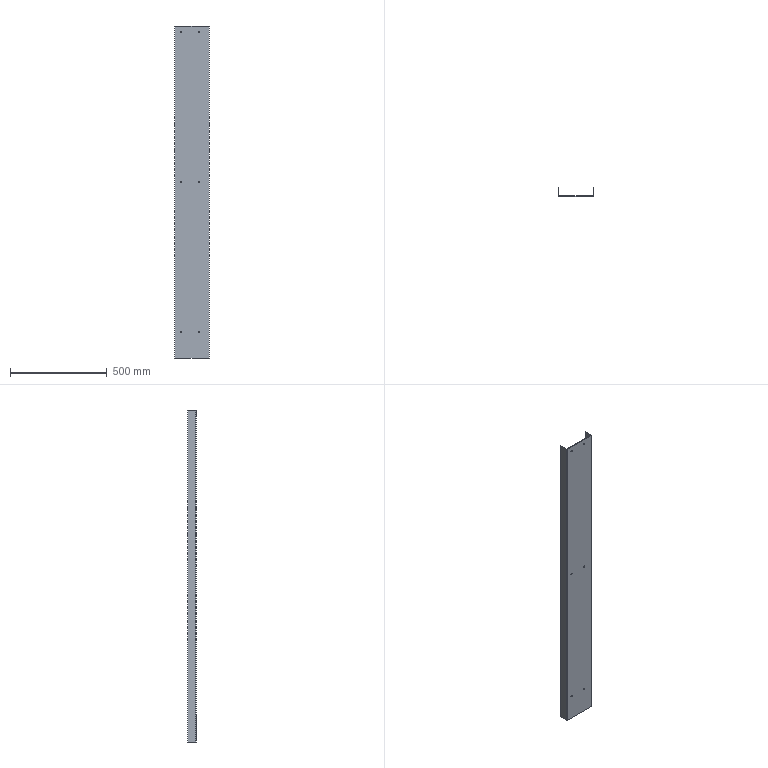Part | SolidWorks | features LPattern 2, Chamfer 1, FlatPattern 1, ICE 1, SMBaseFlange 1, SheetMetal 1 | 1 solid | 46 faces | box 180 x 45 x 1715 mm | volume 683780 mm3 | plane 18 | cylinder 16 | cone 12 | commonest cylinder face diameters 6 x12 1 x2 4 x2
STEP:
#1=CARTESIAN_POINT('',(85.039,61.658,-33.));
#2=VERTEX_POINT('',#1);
#3=CARTESIAN_POINT('',(85.039,61.658,-27.));
#4=VERTEX_POINT('',#3);
#5=CARTESIAN_POINT('',(85.039,61.658,-30.));
#6=DIRECTION('',(0.,1.,0.));
#7=DIRECTION('',(0.,0.,-1.));
#8=AXIS2_PLACEMENT_3D('',#5,#6,#7);
#9=CIRCLE('',#8,3.);
#10=EDGE_CURVE('',#2,#4,#9,.T.);
#11=ORIENTED_EDGE('',*,*,#10,.F.);
#12=CARTESIAN_POINT('',(85.039,62.658,-34.));
#13=VERTEX_POINT('',#12);
#14=CARTESIAN_POINT('',(85.039,61.658,-33.));
#15=DIRECTION('',(0.,0.7071,-0.7071));
#16=VECTOR('',#15,1000.);
#17=LINE('',#14,#16);
#18=EDGE_CURVE('',#2,#13,#17,.T.);
#19=ORIENTED_EDGE('',*,*,#18,.T.);
#20=CARTESIAN_POINT('',(85.039,62.658,-26.));
#21=VERTEX_POINT('',#20);
#22=CARTESIAN_POINT('',(85.039,62.658,-30.));
#23=DIRECTION('',(0.,-1.,0.));
#24=DIRECTION('',(0.,0.,-1.));
#25=AXIS2_PLACEMENT_3D('',#22,#23,#24);
#26=CIRCLE('',#25,4.);
#27=EDGE_CURVE('',#21,#13,#26,.T.);
#28=ORIENTED_EDGE('',*,*,#27,.F.);
#29=CARTESIAN_POINT('',(85.039,61.658,-27.));
#30=DIRECTION('',(0.,0.7071,0.7071));
#31=VECTOR('',#30,1000.);
#32=LINE('',#29,#31);
#33=EDGE_CURVE('',#4,#21,#32,.T.);
#34=ORIENTED_EDGE('',*,*,#33,.F.);
#35=EDGE_LOOP('',(#11,#19,#28,#34));
#36=FACE_OUTER_BOUND('',#35,.T.);
#37=CARTESIAN_POINT('',(85.039,61.658,-30.));
#38=DIRECTION('',(0.,1.,0.));
#39=DIRECTION('',(0.,0.,1.));
#40=AXIS2_PLACEMENT_3D('',#37,#38,#39);
#41=CONICAL_SURFACE('',#40,3.,0.7854);
#42=ADVANCED_FACE('',(#36),#41,.F.);
#43=CARTESIAN_POINT('',(-4.961,61.658,-33.));
#44=VERTEX_POINT('',#43);
#45=CARTESIAN_POINT('',(-4.961,61.658,-27.));
#46=VERTEX_POINT('',#45);
#47=CARTESIAN_POINT('',(-4.961,61.658,-30.));
#48=DIRECTION('',(0.,1.,0.));
#49=DIRECTION('',(0.,0.,-1.));
#50=AXIS2_PLACEMENT_3D('',#47,#48,#49);
#51=CIRCLE('',#50,3.);
#52=EDGE_CURVE('',#44,#46,#51,.T.);
#53=ORIENTED_EDGE('',*,*,#52,.F.);
#54=CARTESIAN_POINT('',(-4.961,62.658,-34.));
#55=VERTEX_POINT('',#54);
#56=CARTESIAN_POINT('',(-4.961,61.658,-33.));
#57=DIRECTION('',(0.,0.7071,-0.7071));
#58=VECTOR('',#57,1000.);
#59=LINE('',#56,#58);
#60=EDGE_CURVE('',#44,#55,#59,.T.);
#61=ORIENTED_EDGE('',*,*,#60,.T.);
#62=CARTESIAN_POINT('',(-4.961,62.658,-26.));
#63=VERTEX_POINT('',#62);
#64=CARTESIAN_POINT('',(-4.961,62.658,-30.));
#65=DIRECTION('',(0.,-1.,0.));
#66=DIRECTION('',(0.,0.,-1.));
#67=AXIS2_PLACEMENT_3D('',#64,#65,#66);
#68=CIRCLE('',#67,4.);
#69=EDGE_CURVE('',#63,#55,#68,.T.);
#70=ORIENTED_EDGE('',*,*,#69,.F.);
#71=CARTESIAN_POINT('',(-4.961,61.658,-27.));
#72=DIRECTION('',(0.,0.7071,0.7071));
#73=VECTOR('',#72,1000.);
#74=LINE('',#71,#73);
#75=EDGE_CURVE('',#46,#63,#74,.T.);
#76=ORIENTED_EDGE('',*,*,#75,.F.);
#77=EDGE_LOOP('',(#53,#61,#70,#76));
#78=FACE_OUTER_BOUND('',#77,.T.);
#79=CARTESIAN_POINT('',(-4.961,61.658,-30.));
#80=DIRECTION('',(0.,1.,0.));
#81=DIRECTION('',(0.,0.,1.));
#82=AXIS2_PLACEMENT_3D('',#79,#80,#81);
#83=CONICAL_SURFACE('',#82,3.,0.7854);
#84=ADVANCED_FACE('',(#78),#83,.F.);
#85=CARTESIAN_POINT('',(85.039,61.158,-27.));
#86=VERTEX_POINT('',#85);
#87=CARTESIAN_POINT('',(85.039,61.158,-33.));
#88=VERTEX_POINT('',#87);
#89=CARTESIAN_POINT('',(85.039,61.158,-30.));
#90=DIRECTION('',(0.,-1.,0.));
#91=DIRECTION('',(0.,0.,-1.));
#92=AXIS2_PLACEMENT_3D('',#89,#90,#91);
#93=CIRCLE('',#92,3.);
#94=EDGE_CURVE('',#86,#88,#93,.T.);
#95=ORIENTED_EDGE('',*,*,#94,.T.);
#96=CARTESIAN_POINT('',(85.039,52.658,-33.));
#97=DIRECTION('',(0.,1.,0.));
#98=VECTOR('',#97,1000.);
#99=LINE('',#96,#98);
#100=EDGE_CURVE('',#88,#2,#99,.T.);
#101=ORIENTED_EDGE('',*,*,#100,.T.);
#102=ORIENTED_EDGE('',*,*,#10,.T.);
#103=CARTESIAN_POINT('',(85.039,52.658,-27.));
#104=DIRECTION('',(0.,1.,0.));
#105=VECTOR('',#104,1000.);
#106=LINE('',#103,#105);
#107=EDGE_CURVE('',#86,#4,#106,.T.);
#108=ORIENTED_EDGE('',*,*,#107,.F.);
#109=EDGE_LOOP('',(#95,#101,#102,#108));
#110=FACE_OUTER_BOUND('',#109,.T.);
#111=CARTESIAN_POINT('',(85.039,52.658,-30.));
#112=DIRECTION('',(0.,1.,0.));
#113=DIRECTION('',(0.,0.,1.));
#114=AXIS2_PLACEMENT_3D('',#111,#112,#113);
#115=CYLINDRICAL_SURFACE('',#114,3.);
#116=ADVANCED_FACE('',(#110),#115,.F.);
#117=CARTESIAN_POINT('',(85.039,61.658,-808.));
#118=VERTEX_POINT('',#117);
#119=CARTESIAN_POINT('',(85.039,61.658,-802.));
#120=VERTEX_POINT('',#119);
#121=CARTESIAN_POINT('',(85.039,61.658,-805.));
#122=DIRECTION('',(0.,1.,0.));
#123=DIRECTION('',(0.,0.,-1.));
#124=AXIS2_PLACEMENT_3D('',#121,#122,#123);
#125=CIRCLE('',#124,3.);
#126=EDGE_CURVE('',#118,#120,#125,.T.);
#127=ORIENTED_EDGE('',*,*,#126,.F.);
#128=CARTESIAN_POINT('',(85.039,62.658,-809.));
#129=VERTEX_POINT('',#128);
#130=CARTESIAN_POINT('',(85.039,61.658,-808.));
#131=DIRECTION('',(0.,0.7071,-0.7071));
#132=VECTOR('',#131,1000.);
#133=LINE('',#130,#132);
#134=EDGE_CURVE('',#118,#129,#133,.T.);
#135=ORIENTED_EDGE('',*,*,#134,.T.);
#136=CARTESIAN_POINT('',(85.039,62.658,-801.));
#137=VERTEX_POINT('',#136);
#138=CARTESIAN_POINT('',(85.039,62.658,-805.));
#139=DIRECTION('',(0.,-1.,0.));
#140=DIRECTION('',(0.,0.,-1.));
#141=AXIS2_PLACEMENT_3D('',#138,#139,#140);
#142=CIRCLE('',#141,4.);
#143=EDGE_CURVE('',#137,#129,#142,.T.);
#144=ORIENTED_EDGE('',*,*,#143,.F.);
#145=CARTESIAN_POINT('',(85.039,61.658,-802.));
#146=DIRECTION('',(0.,0.7071,0.7071));
#147=VECTOR('',#146,1000.);
#148=LINE('',#145,#147);
#149=EDGE_CURVE('',#120,#137,#148,.T.);
#150=ORIENTED_EDGE('',*,*,#149,.F.);
#151=EDGE_LOOP('',(#127,#135,#144,#150));
#152=FACE_OUTER_BOUND('',#151,.T.);
#153=CARTESIAN_POINT('',(85.039,61.658,-805.));
#154=DIRECTION('',(0.,1.,0.));
#155=DIRECTION('',(0.,0.,1.));
#156=AXIS2_PLACEMENT_3D('',#153,#154,#155);
#157=CONICAL_SURFACE('',#156,3.,0.7854);
#158=ADVANCED_FACE('',(#152),#157,.F.);
#159=CARTESIAN_POINT('',(-4.961,61.658,-808.));
#160=VERTEX_POINT('',#159);
#161=CARTESIAN_POINT('',(-4.961,61.658,-802.));
#162=VERTEX_POINT('',#161);
#163=CARTESIAN_POINT('',(-4.961,61.658,-805.));
#164=DIRECTION('',(0.,1.,0.));
#165=DIRECTION('',(0.,0.,-1.));
#166=AXIS2_PLACEMENT_3D('',#163,#164,#165);
#167=CIRCLE('',#166,3.);
#168=EDGE_CURVE('',#160,#162,#167,.T.);
#169=ORIENTED_EDGE('',*,*,#168,.F.);
#170=CARTESIAN_POINT('',(-4.961,62.658,-809.));
#171=VERTEX_POINT('',#170);
#172=CARTESIAN_POINT('',(-4.961,61.658,-808.));
#173=DIRECTION('',(0.,0.7071,-0.7071));
#174=VECTOR('',#173,1000.);
#175=LINE('',#172,#174);
#176=EDGE_CURVE('',#160,#171,#175,.T.);
#177=ORIENTED_EDGE('',*,*,#176,.T.);
#178=CARTESIAN_POINT('',(-4.961,62.658,-801.));
#179=VERTEX_POINT('',#178);
#180=CARTESIAN_POINT('',(-4.961,62.658,-805.));
#181=DIRECTION('',(0.,-1.,0.));
#182=DIRECTION('',(0.,0.,-1.));
#183=AXIS2_PLACEMENT_3D('',#180,#181,#182);
#184=CIRCLE('',#183,4.);
#185=EDGE_CURVE('',#179,#171,#184,.T.);
#186=ORIENTED_EDGE('',*,*,#185,.F.);
#187=CARTESIAN_POINT('',(-4.961,61.658,-802.));
#188=DIRECTION('',(0.,0.7071,0.7071));
#189=VECTOR('',#188,1000.);
#190=LINE('',#187,#189);
#191=EDGE_CURVE('',#162,#179,#190,.T.);
#192=ORIENTED_EDGE('',*,*,#191,.F.);
#193=EDGE_LOOP('',(#169,#177,#186,#192));
#194=FACE_OUTER_BOUND('',#193,.T.);
#195=CARTESIAN_POINT('',(-4.961,61.658,-805.));
#196=DIRECTION('',(0.,1.,0.));
#197=DIRECTION('',(0.,0.,1.));
#198=AXIS2_PLACEMENT_3D('',#195,#196,#197);
#199=CONICAL_SURFACE('',#198,3.,0.7854);
#200=ADVANCED_FACE('',(#194),#199,.F.);
#201=CARTESIAN_POINT('',(85.039,61.158,-802.));
#202=VERTEX_POINT('',#201);
#203=CARTESIAN_POINT('',(85.039,61.158,-808.));
#204=VERTEX_POINT('',#203);
#205=CARTESIAN_POINT('',(85.039,61.158,-805.));
#206=DIRECTION('',(0.,-1.,0.));
#207=DIRECTION('',(0.,0.,-1.));
#208=AXIS2_PLACEMENT_3D('',#205,#206,#207);
#209=CIRCLE('',#208,3.);
#210=EDGE_CURVE('',#202,#204,#209,.T.);
#211=ORIENTED_EDGE('',*,*,#210,.T.);
#212=CARTESIAN_POINT('',(85.039,52.658,-808.));
#213=DIRECTION('',(0.,1.,0.));
#214=VECTOR('',#213,1000.);
#215=LINE('',#212,#214);
#216=EDGE_CURVE('',#204,#118,#215,.T.);
#217=ORIENTED_EDGE('',*,*,#216,.T.);
#218=ORIENTED_EDGE('',*,*,#126,.T.);
#219=CARTESIAN_POINT('',(85.039,52.658,-802.));
#220=DIRECTION('',(0.,1.,0.));
#221=VECTOR('',#220,1000.);
#222=LINE('',#219,#221);
#223=EDGE_CURVE('',#202,#120,#222,.T.);
#224=ORIENTED_EDGE('',*,*,#223,.F.);
#225=EDGE_LOOP('',(#211,#217,#218,#224));
#226=FACE_OUTER_BOUND('',#225,.T.);
#227=CARTESIAN_POINT('',(85.039,52.658,-805.));
#228=DIRECTION('',(0.,1.,0.));
#229=DIRECTION('',(0.,0.,1.));
#230=AXIS2_PLACEMENT_3D('',#227,#228,#229);
#231=CYLINDRICAL_SURFACE('',#230,3.);
#232=ADVANCED_FACE('',(#226),#231,.F.);
#233=CARTESIAN_POINT('',(-4.961,61.158,-27.));
#234=VERTEX_POINT('',#233);
#235=CARTESIAN_POINT('',(-4.961,61.158,-33.));
#236=VERTEX_POINT('',#235);
#237=CARTESIAN_POINT('',(-4.961,61.158,-30.));
#238=DIRECTION('',(0.,-1.,0.));
#239=DIRECTION('',(0.,0.,-1.));
#240=AXIS2_PLACEMENT_3D('',#237,#238,#239);
#241=CIRCLE('',#240,3.);
#242=EDGE_CURVE('',#234,#236,#241,.T.);
#243=ORIENTED_EDGE('',*,*,#242,.T.);
#244=CARTESIAN_POINT('',(-4.961,52.658,-33.));
#245=DIRECTION('',(0.,1.,0.));
#246=VECTOR('',#245,1000.);
#247=LINE('',#244,#246);
#248=EDGE_CURVE('',#236,#44,#247,.T.);
#249=ORIENTED_EDGE('',*,*,#248,.T.);
#250=ORIENTED_EDGE('',*,*,#52,.T.);
#251=CARTESIAN_POINT('',(-4.961,52.658,-27.));
#252=DIRECTION('',(0.,1.,0.));
#253=VECTOR('',#252,1000.);
#254=LINE('',#251,#253);
#255=EDGE_CURVE('',#234,#46,#254,.T.);
#256=ORIENTED_EDGE('',*,*,#255,.F.);
#257=EDGE_LOOP('',(#243,#249,#250,#256));
#258=FACE_OUTER_BOUND('',#257,.T.);
#259=CARTESIAN_POINT('',(-4.961,52.658,-30.));
#260=DIRECTION('',(0.,1.,0.));
#261=DIRECTION('',(0.,0.,1.));
#262=AXIS2_PLACEMENT_3D('',#259,#260,#261);
#263=CYLINDRICAL_SURFACE('',#262,3.);
#264=ADVANCED_FACE('',(#258),#263,.F.);
#265=CARTESIAN_POINT('',(-4.961,61.158,-802.));
#266=VERTEX_POINT('',#265);
#267=CARTESIAN_POINT('',(-4.961,61.158,-808.));
#268=VERTEX_POINT('',#267);
#269=CARTESIAN_POINT('',(-4.961,61.158,-805.));
#270=DIRECTION('',(0.,-1.,0.));
#271=DIRECTION('',(0.,0.,-1.));
#272=AXIS2_PLACEMENT_3D('',#269,#270,#271);
#273=CIRCLE('',#272,3.);
#274=EDGE_CURVE('',#266,#268,#273,.T.);
#275=ORIENTED_EDGE('',*,*,#274,.T.);
#276=CARTESIAN_POINT('',(-4.961,52.658,-808.));
#277=DIRECTION('',(0.,1.,0.));
#278=VECTOR('',#277,1000.);
#279=LINE('',#276,#278);
#280=EDGE_CURVE('',#268,#160,#279,.T.);
#281=ORIENTED_EDGE('',*,*,#280,.T.);
#282=ORIENTED_EDGE('',*,*,#168,.T.);
#283=CARTESIAN_POINT('',(-4.961,52.658,-802.));
#284=DIRECTION('',(0.,1.,0.));
#285=VECTOR('',#284,1000.);
#286=LINE('',#283,#285);
#287=EDGE_CURVE('',#266,#162,#286,.T.);
#288=ORIENTED_EDGE('',*,*,#287,.F.);
#289=EDGE_LOOP('',(#275,#281,#282,#288));
#290=FACE_OUTER_BOUND('',#289,.T.);
#291=CARTESIAN_POINT('',(-4.961,52.658,-805.));
#292=DIRECTION('',(0.,1.,0.));
#293=DIRECTION('',(0.,0.,1.));
#294=AXIS2_PLACEMENT_3D('',#291,#292,#293);
#295=CYLINDRICAL_SURFACE('',#294,3.);
#296=ADVANCED_FACE('',(#290),#295,.F.);
#297=CARTESIAN_POINT('',(85.039,61.658,-1583.));
#298=VERTEX_POINT('',#297);
#299=CARTESIAN_POINT('',(85.039,61.658,-1577.));
#300=VERTEX_POINT('',#299);
#301=CARTESIAN_POINT('',(85.039,61.658,-1580.));
#302=DIRECTION('',(0.,1.,0.));
#303=DIRECTION('',(0.,0.,-1.));
#304=AXIS2_PLACEMENT_3D('',#301,#302,#303);
#305=CIRCLE('',#304,3.);
#306=EDGE_CURVE('',#298,#300,#305,.T.);
#307=ORIENTED_EDGE('',*,*,#306,.F.);
#308=CARTESIAN_POINT('',(85.039,62.658,-1584.));
#309=VERTEX_POINT('',#308);
#310=CARTESIAN_POINT('',(85.039,61.658,-1583.));
#311=DIRECTION('',(0.,0.7071,-0.7071));
#312=VECTOR('',#311,1000.);
#313=LINE('',#310,#312);
#314=EDGE_CURVE('',#298,#309,#313,.T.);
#315=ORIENTED_EDGE('',*,*,#314,.T.);
#316=CARTESIAN_POINT('',(85.039,62.658,-1576.));
#317=VERTEX_POINT('',#316);
#318=CARTESIAN_POINT('',(85.039,62.658,-1580.));
#319=DIRECTION('',(0.,-1.,0.));
#320=DIRECTION('',(0.,0.,-1.));
#321=AXIS2_PLACEMENT_3D('',#318,#319,#320);
#322=CIRCLE('',#321,4.);
#323=EDGE_CURVE('',#317,#309,#322,.T.);
#324=ORIENTED_EDGE('',*,*,#323,.F.);
#325=CARTESIAN_POINT('',(85.039,61.658,-1577.));
#326=DIRECTION('',(0.,0.7071,0.7071));
#327=VECTOR('',#326,1000.);
#328=LINE('',#325,#327);
#329=EDGE_CURVE('',#300,#317,#328,.T.);
#330=ORIENTED_EDGE('',*,*,#329,.F.);
#331=EDGE_LOOP('',(#307,#315,#324,#330));
#332=FACE_OUTER_BOUND('',#331,.T.);
#333=CARTESIAN_POINT('',(85.039,61.658,-1580.));
#334=DIRECTION('',(0.,1.,0.));
#335=DIRECTION('',(0.,0.,1.));
#336=AXIS2_PLACEMENT_3D('',#333,#334,#335);
#337=CONICAL_SURFACE('',#336,3.,0.7854);
#338=ADVANCED_FACE('',(#332),#337,.F.);
#339=CARTESIAN_POINT('',(85.039,61.158,-1577.));
#340=VERTEX_POINT('',#339);
#341=CARTESIAN_POINT('',(85.039,61.158,-1583.));
#342=VERTEX_POINT('',#341);
#343=CARTESIAN_POINT('',(85.039,61.158,-1580.));
#344=DIRECTION('',(0.,-1.,0.));
#345=DIRECTION('',(0.,0.,-1.));
#346=AXIS2_PLACEMENT_3D('',#343,#344,#345);
#347=CIRCLE('',#346,3.);
#348=EDGE_CURVE('',#340,#342,#347,.T.);
#349=ORIENTED_EDGE('',*,*,#348,.T.);
#350=CARTESIAN_POINT('',(85.039,52.658,-1583.));
#351=DIRECTION('',(0.,1.,0.));
#352=VECTOR('',#351,1000.);
#353=LINE('',#350,#352);
#354=EDGE_CURVE('',#342,#298,#353,.T.);
#355=ORIENTED_EDGE('',*,*,#354,.T.);
#356=ORIENTED_EDGE('',*,*,#306,.T.);
#357=CARTESIAN_POINT('',(85.039,52.658,-1577.));
#358=DIRECTION('',(0.,1.,0.));
#359=VECTOR('',#358,1000.);
#360=LINE('',#357,#359);
#361=EDGE_CURVE('',#340,#300,#360,.T.);
#362=ORIENTED_EDGE('',*,*,#361,.F.);
#363=EDGE_LOOP('',(#349,#355,#356,#362));
#364=FACE_OUTER_BOUND('',#363,.T.);
#365=CARTESIAN_POINT('',(85.039,52.658,-1580.));
#366=DIRECTION('',(0.,1.,0.));
#367=DIRECTION('',(0.,0.,1.));
#368=AXIS2_PLACEMENT_3D('',#365,#366,#367);
#369=CYLINDRICAL_SURFACE('',#368,3.);
#370=ADVANCED_FACE('',(#364),#369,.F.);
#371=CARTESIAN_POINT('',(-4.961,61.658,-1583.));
#372=VERTEX_POINT('',#371);
#373=CARTESIAN_POINT('',(-4.961,61.658,-1577.));
#374=VERTEX_POINT('',#373);
#375=CARTESIAN_POINT('',(-4.961,61.658,-1580.));
#376=DIRECTION('',(0.,1.,0.));
#377=DIRECTION('',(0.,0.,-1.));
#378=AXIS2_PLACEMENT_3D('',#375,#376,#377);
#379=CIRCLE('',#378,3.);
#380=EDGE_CURVE('',#372,#374,#379,.T.);
#381=ORIENTED_EDGE('',*,*,#380,.F.);
#382=CARTESIAN_POINT('',(-4.961,62.658,-1584.));
#383=VERTEX_POINT('',#382);
#384=CARTESIAN_POINT('',(-4.961,61.658,-1583.));
#385=DIRECTION('',(0.,0.7071,-0.7071));
#386=VECTOR('',#385,1000.);
#387=LINE('',#384,#386);
#388=EDGE_CURVE('',#372,#383,#387,.T.);
#389=ORIENTED_EDGE('',*,*,#388,.T.);
#390=CARTESIAN_POINT('',(-4.961,62.658,-1576.));
#391=VERTEX_POINT('',#390);
#392=CARTESIAN_POINT('',(-4.961,62.658,-1580.));
#393=DIRECTION('',(0.,-1.,0.));
#394=DIRECTION('',(0.,0.,-1.));
#395=AXIS2_PLACEMENT_3D('',#392,#393,#394);
#396=CIRCLE('',#395,4.);
#397=EDGE_CURVE('',#391,#383,#396,.T.);
#398=ORIENTED_EDGE('',*,*,#397,.F.);
#399=CARTESIAN_POINT('',(-4.961,61.658,-1577.));
#400=DIRECTION('',(0.,0.7071,0.7071));
#401=VECTOR('',#400,1000.);
#402=LINE('',#399,#401);
#403=EDGE_CURVE('',#374,#391,#402,.T.);
#404=ORIENTED_EDGE('',*,*,#403,.F.);
#405=EDGE_LOOP('',(#381,#389,#398,#404));
#406=FACE_OUTER_BOUND('',#405,.T.);
#407=CARTESIAN_POINT('',(-4.961,61.658,-1580.));
#408=DIRECTION('',(0.,1.,0.));
#409=DIRECTION('',(0.,0.,1.));
#410=AXIS2_PLACEMENT_3D('',#407,#408,#409);
#411=CONICAL_SURFACE('',#410,3.,0.7854);
#412=ADVANCED_FACE('',(#406),#411,.F.);
#413=CARTESIAN_POINT('',(-4.961,61.158,-1577.));
#414=VERTEX_POINT('',#413);
#415=CARTESIAN_POINT('',(-4.961,61.158,-1583.));
#416=VERTEX_POINT('',#415);
#417=CARTESIAN_POINT('',(-4.961,61.158,-1580.));
#418=DIRECTION('',(0.,-1.,0.));
#419=DIRECTION('',(0.,0.,-1.));
#420=AXIS2_PLACEMENT_3D('',#417,#418,#419);
#421=CIRCLE('',#420,3.);
#422=EDGE_CURVE('',#414,#416,#421,.T.);
#423=ORIENTED_EDGE('',*,*,#422,.T.);
#424=CARTESIAN_POINT('',(-4.961,52.658,-1583.));
#425=DIRECTION('',(0.,1.,0.));
#426=VECTOR('',#425,1000.);
#427=LINE('',#424,#426);
#428=EDGE_CURVE('',#416,#372,#427,.T.);
#429=ORIENTED_EDGE('',*,*,#428,.T.);
#430=ORIENTED_EDGE('',*,*,#380,.T.);
#431=CARTESIAN_POINT('',(-4.961,52.658,-1577.));
#432=DIRECTION('',(0.,1.,0.));
#433=VECTOR('',#432,1000.);
#434=LINE('',#431,#433);
#435=EDGE_CURVE('',#414,#374,#434,.T.);
#436=ORIENTED_EDGE('',*,*,#435,.F.);
#437=EDGE_LOOP('',(#423,#429,#430,#436));
#438=FACE_OUTER_BOUND('',#437,.T.);
#439=CARTESIAN_POINT('',(-4.961,52.658,-1580.));
#440=DIRECTION('',(0.,1.,0.));
#441=DIRECTION('',(0.,0.,1.));
#442=AXIS2_PLACEMENT_3D('',#439,#440,#441);
#443=CYLINDRICAL_SURFACE('',#442,3.);
#444=ADVANCED_FACE('',(#438),#443,.F.);
#445=CARTESIAN_POINT('',(-37.961,61.158,-1715.));
#446=VERTEX_POINT('',#445);
#447=CARTESIAN_POINT('',(-37.961,62.658,-1715.));
#448=VERTEX_POINT('',#447);
#449=CARTESIAN_POINT('',(-37.961,61.158,-1715.));
#450=DIRECTION('',(0.,1.,0.));
#451=VECTOR('',#450,1000.);
#452=LINE('',#449,#451);
#453=EDGE_CURVE('',#446,#448,#452,.T.);
#454=ORIENTED_EDGE('',*,*,#453,.F.);
#455=CARTESIAN_POINT('',(-39.961,63.158,-1715.));
#456=VERTEX_POINT('',#455);
#457=CARTESIAN_POINT('',(-37.961,63.158,-1715.));
#458=DIRECTION('',(0.,0.,1.));
#459=DIRECTION('',(-1.,0.,0.));
#460=AXIS2_PLACEMENT_3D('',#457,#458,#459);
#461=CIRCLE('',#460,2.);
#462=EDGE_CURVE('',#456,#446,#461,.T.);
#463=ORIENTED_EDGE('',*,*,#462,.F.);
#464=CARTESIAN_POINT('',(-38.461,63.158,-1715.));
#465=VERTEX_POINT('',#464);
#466=CARTESIAN_POINT('',(-38.461,63.158,-1715.));
#467=DIRECTION('',(-1.,0.,0.));
#468=VECTOR('',#467,1000.);
#469=LINE('',#466,#468);
#470=EDGE_CURVE('',#465,#456,#469,.T.);
#471=ORIENTED_EDGE('',*,*,#470,.F.);
#472=CARTESIAN_POINT('',(-37.961,63.158,-1715.));
#473=DIRECTION('',(0.,0.,1.));
#474=DIRECTION('',(1.,0.,0.));
#475=AXIS2_PLACEMENT_3D('',#472,#473,#474);
#476=CIRCLE('',#475,0.5);
#477=EDGE_CURVE('',#465,#448,#476,.T.);
#478=ORIENTED_EDGE('',*,*,#477,.T.);
#479=EDGE_LOOP('',(#454,#463,#471,#478));
#480=FACE_OUTER_BOUND('',#479,.T.);
#481=CARTESIAN_POINT('',(-37.961,61.158,-1715.));
#482=DIRECTION('',(0.,0.,-1.));
#483=DIRECTION('',(-1.,0.,0.));
#484=AXIS2_PLACEMENT_3D('',#481,#482,#483);
#485=PLANE('',#484);
#486=ADVANCED_FACE('',(#480),#485,.T.);
#487=CARTESIAN_POINT('',(138.039,61.158,-1715.));
#488=VERTEX_POINT('',#487);
#489=CARTESIAN_POINT('',(-39.961,61.158,-1715.));
#490=DIRECTION('',(1.,0.,0.));
#491=VECTOR('',#490,1000.);
#492=LINE('',#489,#491);
#493=EDGE_CURVE('',#446,#488,#492,.T.);
#494=ORIENTED_EDGE('',*,*,#493,.F.);
#495=ORIENTED_EDGE('',*,*,#453,.T.);
#496=CARTESIAN_POINT('',(138.039,62.658,-1715.));
#497=VERTEX_POINT('',#496);
#498=CARTESIAN_POINT('',(-39.961,62.658,-1715.));
#499=DIRECTION('',(1.,0.,0.));
#500=VECTOR('',#499,1000.);
#501=LINE('',#498,#500);
#502=EDGE_CURVE('',#448,#497,#501,.T.);
#503=ORIENTED_EDGE('',*,*,#502,.T.);
#504=CARTESIAN_POINT('',(138.039,62.658,-1715.));
#505=DIRECTION('',(0.,-1.,0.));
#506=VECTOR('',#505,1000.);
#507=LINE('',#504,#506);
#508=EDGE_CURVE('',#497,#488,#507,.T.);
#509=ORIENTED_EDGE('',*,*,#508,.T.);
#510=EDGE_LOOP('',(#494,#495,#503,#509));
#511=FACE_OUTER_BOUND('',#510,.T.);
#512=CARTESIAN_POINT('',(-38.461,63.158,-1715.));
#513=DIRECTION('',(0.,0.,-1.));
#514=DIRECTION('',(-1.,0.,0.));
#515=AXIS2_PLACEMENT_3D('',#512,#513,#514);
#516=PLANE('',#515);
#517=ADVANCED_FACE('',(#511),#516,.T.);
#518=CARTESIAN_POINT('',(-39.961,63.158,0.));
#519=VERTEX_POINT('',#518);
#520=CARTESIAN_POINT('',(-38.461,63.158,0.));
#521=VERTEX_POINT('',#520);
#522=CARTESIAN_POINT('',(-39.961,63.158,0.));
#523=DIRECTION('',(1.,0.,0.));
#524=VECTOR('',#523,1000.);
#525=LINE('',#522,#524);
#526=EDGE_CURVE('',#519,#521,#525,.T.);
#527=ORIENTED_EDGE('',*,*,#526,.F.);
#528=CARTESIAN_POINT('',(-37.961,61.158,0.));
#529=VERTEX_POINT('',#528);
#530=CARTESIAN_POINT('',(-37.961,63.158,0.));
#531=DIRECTION('',(0.,0.,1.));
#532=DIRECTION('',(-1.,0.,0.));
#533=AXIS2_PLACEMENT_3D('',#530,#531,#532);
#534=CIRCLE('',#533,2.);
#535=EDGE_CURVE('',#519,#529,#534,.T.);
#536=ORIENTED_EDGE('',*,*,#535,.T.);
#537=CARTESIAN_POINT('',(-37.961,62.658,0.));
#538=VERTEX_POINT('',#537);
#539=CARTESIAN_POINT('',(-37.961,62.658,0.));
#540=DIRECTION('',(0.,-1.,0.));
#541=VECTOR('',#540,1000.);
#542=LINE('',#539,#541);
#543=EDGE_CURVE('',#538,#529,#542,.T.);
#544=ORIENTED_EDGE('',*,*,#543,.F.);
#545=CARTESIAN_POINT('',(-37.961,63.158,0.));
#546=DIRECTION('',(0.,0.,1.));
#547=DIRECTION('',(1.,0.,0.));
#548=AXIS2_PLACEMENT_3D('',#545,#546,#547);
#549=CIRCLE('',#548,0.5);
#550=EDGE_CURVE('',#521,#538,#549,.T.);
#551=ORIENTED_EDGE('',*,*,#550,.F.);
#552=EDGE_LOOP('',(#527,#536,#544,#551));
#553=FACE_OUTER_BOUND('',#552,.T.);
#554=CARTESIAN_POINT('',(-39.961,63.158,0.));
#555=DIRECTION('',(0.,0.,1.));
#556=DIRECTION('',(1.,0.,0.));
#557=AXIS2_PLACEMENT_3D('',#554,#555,#556);
#558=PLANE('',#557);
#559=ADVANCED_FACE('',(#553),#558,.T.);
#560=CARTESIAN_POINT('',(-39.961,106.158,0.));
#561=VERTEX_POINT('',#560);
#562=CARTESIAN_POINT('',(-39.961,106.158,0.));
#563=DIRECTION('',(0.,-1.,0.));
#564=VECTOR('',#563,1000.);
#565=LINE('',#562,#564);
#566=EDGE_CURVE('',#561,#519,#565,.T.);
#567=ORIENTED_EDGE('',*,*,#566,.T.);
#568=ORIENTED_EDGE('',*,*,#526,.T.);
#569=CARTESIAN_POINT('',(-38.461,106.158,0.));
#570=VERTEX_POINT('',#569);
#571=CARTESIAN_POINT('',(-38.461,106.158,0.));
#572=DIRECTION('',(0.,-1.,0.));
#573=VECTOR('',#572,1000.);
#574=LINE('',#571,#573);
#575=EDGE_CURVE('',#570,#521,#574,.T.);
#576=ORIENTED_EDGE('',*,*,#575,.F.);
#577=CARTESIAN_POINT('',(-39.961,106.158,0.));
#578=DIRECTION('',(1.,0.,0.));
#579=VECTOR('',#578,1000.);
#580=LINE('',#577,#579);
#581=EDGE_CURVE('',#561,#570,#580,.T.);
#582=ORIENTED_EDGE('',*,*,#581,.F.);
#583=EDGE_LOOP('',(#567,#568,#576,#582));
#584=FACE_OUTER_BOUND('',#583,.T.);
#585=CARTESIAN_POINT('',(-37.961,62.658,0.));
#586=DIRECTION('',(0.,0.,1.));
#587=DIRECTION('',(1.,0.,0.));
#588=AXIS2_PLACEMENT_3D('',#585,#586,#587);
#589=PLANE('',#588);
#590=ADVANCED_FACE('',(#584),#589,.T.);
#591=CARTESIAN_POINT('',(140.039,63.158,-1715.));
#592=VERTEX_POINT('',#591);
#593=CARTESIAN_POINT('',(138.539,63.158,-1715.));
#594=VERTEX_POINT('',#593);
#595=CARTESIAN_POINT('',(140.039,63.158,-1715.));
#596=DIRECTION('',(-1.,0.,0.));
#597=VECTOR('',#596,1000.);
#598=LINE('',#595,#597);
#599=EDGE_CURVE('',#592,#594,#598,.T.);
#600=ORIENTED_EDGE('',*,*,#599,.F.);
#601=CARTESIAN_POINT('',(138.039,63.158,-1715.));
#602=DIRECTION('',(0.,0.,1.));
#603=DIRECTION('',(-1.,0.,0.));
#604=AXIS2_PLACEMENT_3D('',#601,#602,#603);
#605=CIRCLE('',#604,2.);
#606=EDGE_CURVE('',#488,#592,#605,.T.);
#607=ORIENTED_EDGE('',*,*,#606,.F.);
#608=ORIENTED_EDGE('',*,*,#508,.F.);
#609=CARTESIAN_POINT('',(138.039,63.158,-1715.));
#610=DIRECTION('',(0.,0.,1.));
#611=DIRECTION('',(1.,0.,0.));
#612=AXIS2_PLACEMENT_3D('',#609,#610,#611);
#613=CIRCLE('',#612,0.5);
#614=EDGE_CURVE('',#497,#594,#613,.T.);
#615=ORIENTED_EDGE('',*,*,#614,.T.);
#616=EDGE_LOOP('',(#600,#607,#608,#615));
#617=FACE_OUTER_BOUND('',#616,.T.);
#618=CARTESIAN_POINT('',(140.039,63.158,-1715.));
#619=DIRECTION('',(0.,0.,-1.));
#620=DIRECTION('',(-1.,0.,0.));
#621=AXIS2_PLACEMENT_3D('',#618,#619,#620);
#622=PLANE('',#621);
#623=ADVANCED_FACE('',(#617),#622,.T.);
#624=CARTESIAN_POINT('',(140.039,106.158,-1715.));
#625=VERTEX_POINT('',#624);
#626=CARTESIAN_POINT('',(140.039,61.158,-1715.));
#627=DIRECTION('',(0.,1.,0.));
#628=VECTOR('',#627,1000.);
#629=LINE('',#626,#628);
#630=EDGE_CURVE('',#592,#625,#629,.T.);
#631=ORIENTED_EDGE('',*,*,#630,.F.);
#632=ORIENTED_EDGE('',*,*,#599,.T.);
#633=CARTESIAN_POINT('',(138.539,106.158,-1715.));
#634=VERTEX_POINT('',#633);
#635=CARTESIAN_POINT('',(138.539,61.158,-1715.));
#636=DIRECTION('',(0.,1.,0.));
#637=VECTOR('',#636,1000.);
#638=LINE('',#635,#637);
#639=EDGE_CURVE('',#594,#634,#638,.T.);
#640=ORIENTED_EDGE('',*,*,#639,.T.);
#641=CARTESIAN_POINT('',(138.539,106.158,-1715.));
#642=DIRECTION('',(1.,0.,0.));
#643=VECTOR('',#642,1000.);
#644=LINE('',#641,#643);
#645=EDGE_CURVE('',#634,#625,#644,.T.);
#646=ORIENTED_EDGE('',*,*,#645,.T.);
#647=EDGE_LOOP('',(#631,#632,#640,#646));
#648=FACE_OUTER_BOUND('',#647,.T.);
#649=CARTESIAN_POINT('',(138.039,62.658,-1715.));
#650=DIRECTION('',(0.,0.,-1.));
#651=DIRECTION('',(-1.,0.,0.));
#652=AXIS2_PLACEMENT_3D('',#649,#650,#651);
#653=PLANE('',#652);
#654=ADVANCED_FACE('',(#648),#653,.T.);
#655=CARTESIAN_POINT('',(138.039,61.158,0.));
#656=VERTEX_POINT('',#655);
#657=CARTESIAN_POINT('',(138.039,62.658,0.));
#658=VERTEX_POINT('',#657);
#659=CARTESIAN_POINT('',(138.039,61.158,0.));
#660=DIRECTION('',(0.,1.,0.));
#661=VECTOR('',#660,1000.);
#662=LINE('',#659,#661);
#663=EDGE_CURVE('',#656,#658,#662,.T.);
#664=ORIENTED_EDGE('',*,*,#663,.F.);
#665=CARTESIAN_POINT('',(140.039,63.158,0.));
#666=VERTEX_POINT('',#665);
#667=CARTESIAN_POINT('',(138.039,63.158,0.));
#668=DIRECTION('',(0.,0.,1.));
#669=DIRECTION('',(-1.,0.,0.));
#670=AXIS2_PLACEMENT_3D('',#667,#668,#669);
#671=CIRCLE('',#670,2.);
#672=EDGE_CURVE('',#656,#666,#671,.T.);
#673=ORIENTED_EDGE('',*,*,#672,.T.);
#674=CARTESIAN_POINT('',(138.539,63.158,0.));
#675=VERTEX_POINT('',#674);
#676=CARTESIAN_POINT('',(138.539,63.158,0.));
#677=DIRECTION('',(1.,0.,0.));
#678=VECTOR('',#677,1000.);
#679=LINE('',#676,#678);
#680=EDGE_CURVE('',#675,#666,#679,.T.);
#681=ORIENTED_EDGE('',*,*,#680,.F.);
#682=CARTESIAN_POINT('',(138.039,63.158,0.));
#683=DIRECTION('',(0.,0.,1.));
#684=DIRECTION('',(1.,0.,0.));
#685=AXIS2_PLACEMENT_3D('',#682,#683,#684);
#686=CIRCLE('',#685,0.5);
#687=EDGE_CURVE('',#658,#675,#686,.T.);
#688=ORIENTED_EDGE('',*,*,#687,.F.);
#689=EDGE_LOOP('',(#664,#673,#681,#688));
#690=FACE_OUTER_BOUND('',#689,.T.);
#691=CARTESIAN_POINT('',(138.039,61.158,0.));
#692=DIRECTION('',(0.,0.,1.));
#693=DIRECTION('',(1.,0.,0.));
#694=AXIS2_PLACEMENT_3D('',#691,#692,#693);
#695=PLANE('',#694);
#696=ADVANCED_FACE('',(#690),#695,.T.);
#697=CARTESIAN_POINT('',(-39.961,61.158,0.));
#698=DIRECTION('',(1.,0.,0.));
#699=VECTOR('',#698,1000.);
#700=LINE('',#697,#699);
#701=EDGE_CURVE('',#529,#656,#700,.T.);
#702=ORIENTED_EDGE('',*,*,#701,.T.);
#703=ORIENTED_EDGE('',*,*,#663,.T.);
#704=CARTESIAN_POINT('',(-39.961,62.658,0.));
#705=DIRECTION('',(1.,0.,0.));
#706=VECTOR('',#705,1000.);
#707=LINE('',#704,#706);
#708=EDGE_CURVE('',#538,#658,#707,.T.);
#709=ORIENTED_EDGE('',*,*,#708,.F.);
#710=ORIENTED_EDGE('',*,*,#543,.T.);
#711=EDGE_LOOP('',(#702,#703,#709,#710));
#712=FACE_OUTER_BOUND('',#711,.T.);
#713=CARTESIAN_POINT('',(138.539,63.158,0.));
#714=DIRECTION('',(0.,0.,1.));
#715=DIRECTION('',(1.,0.,0.));
#716=AXIS2_PLACEMENT_3D('',#713,#714,#715);
#717=PLANE('',#716);
#718=ADVANCED_FACE('',(#712),#717,.T.);
#719=CARTESIAN_POINT('',(140.039,106.158,0.));
#720=VERTEX_POINT('',#719);
#721=CARTESIAN_POINT('',(140.039,61.158,0.));
#722=DIRECTION('',(0.,1.,0.));
#723=VECTOR('',#722,1000.);
#724=LINE('',#721,#723);
#725=EDGE_CURVE('',#666,#720,#724,.T.);
#726=ORIENTED_EDGE('',*,*,#725,.F.);
#727=CARTESIAN_POINT('',(140.039,63.158,-1715.));
#728=DIRECTION('',(0.,0.,1.));
#729=VECTOR('',#728,1000.);
#730=LINE('',#727,#729);
#731=EDGE_CURVE('',#592,#666,#730,.T.);
#732=ORIENTED_EDGE('',*,*,#731,.F.);
#733=ORIENTED_EDGE('',*,*,#630,.T.);
#734=CARTESIAN_POINT('',(140.039,106.158,-1715.));
#735=DIRECTION('',(0.,0.,1.));
#736=VECTOR('',#735,1000.);
#737=LINE('',#734,#736);
#738=EDGE_CURVE('',#625,#720,#737,.T.);
#739=ORIENTED_EDGE('',*,*,#738,.T.);
#740=EDGE_LOOP('',(#726,#732,#733,#739));
#741=FACE_OUTER_BOUND('',#740,.T.);
#742=CARTESIAN_POINT('',(140.039,61.158,-1715.));
#743=DIRECTION('',(1.,0.,0.));
#744=DIRECTION('',(0.,0.,-1.));
#745=AXIS2_PLACEMENT_3D('',#742,#743,#744);
#746=PLANE('',#745);
#747=ADVANCED_FACE('',(#741),#746,.T.);
#748=ORIENTED_EDGE('',*,*,#672,.F.);
#749=CARTESIAN_POINT('',(138.039,61.158,-1715.));
#750=DIRECTION('',(0.,0.,1.));
#751=VECTOR('',#750,1000.);
#752=LINE('',#749,#751);
#753=EDGE_CURVE('',#488,#656,#752,.T.);
#754=ORIENTED_EDGE('',*,*,#753,.F.);
#755=ORIENTED_EDGE('',*,*,#606,.T.);
#756=ORIENTED_EDGE('',*,*,#731,.T.);
#757=EDGE_LOOP('',(#748,#754,#755,#756));
#758=FACE_OUTER_BOUND('',#757,.T.);
#759=CARTESIAN_POINT('',(138.039,63.158,-1715.));
#760=DIRECTION('',(0.,0.,1.));
#761=DIRECTION('',(1.,0.,0.));
#762=AXIS2_PLACEMENT_3D('',#759,#760,#761);
#763=CYLINDRICAL_SURFACE('',#762,2.);
#764=ADVANCED_FACE('',(#758),#763,.T.);
#765=ORIENTED_EDGE('',*,*,#94,.F.);
#766=CARTESIAN_POINT('',(85.039,61.158,-30.));
#767=DIRECTION('',(0.,-1.,0.));
#768=DIRECTION('',(0.,0.,-1.));
#769=AXIS2_PLACEMENT_3D('',#766,#767,#768);
#770=CIRCLE('',#769,3.);
#771=EDGE_CURVE('',#88,#86,#770,.T.);
#772=ORIENTED_EDGE('',*,*,#771,.F.);
#773=EDGE_LOOP('',(#765,#772));
#774=FACE_BOUND('',#773,.T.);
#775=ORIENTED_EDGE('',*,*,#210,.F.);
#776=CARTESIAN_POINT('',(85.039,61.158,-805.));
#777=DIRECTION('',(0.,-1.,0.));
#778=DIRECTION('',(0.,0.,-1.));
#779=AXIS2_PLACEMENT_3D('',#776,#777,#778);
#780=CIRCLE('',#779,3.);
#781=EDGE_CURVE('',#204,#202,#780,.T.);
#782=ORIENTED_EDGE('',*,*,#781,.F.);
#783=EDGE_LOOP('',(#775,#782));
#784=FACE_BOUND('',#783,.T.);
#785=ORIENTED_EDGE('',*,*,#242,.F.);
#786=CARTESIAN_POINT('',(-4.961,61.158,-30.));
#787=DIRECTION('',(0.,-1.,0.));
#788=DIRECTION('',(0.,0.,-1.));
#789=AXIS2_PLACEMENT_3D('',#786,#787,#788);
#790=CIRCLE('',#789,3.);
#791=EDGE_CURVE('',#236,#234,#790,.T.);
#792=ORIENTED_EDGE('',*,*,#791,.F.);
#793=EDGE_LOOP('',(#785,#792));
#794=FACE_BOUND('',#793,.T.);
#795=ORIENTED_EDGE('',*,*,#274,.F.);
#796=CARTESIAN_POINT('',(-4.961,61.158,-805.));
#797=DIRECTION('',(0.,-1.,0.));
#798=DIRECTION('',(0.,0.,-1.));
#799=AXIS2_PLACEMENT_3D('',#796,#797,#798);
#800=CIRCLE('',#799,3.);
#801=EDGE_CURVE('',#268,#266,#800,.T.);
#802=ORIENTED_EDGE('',*,*,#801,.F.);
#803=EDGE_LOOP('',(#795,#802));
#804=FACE_BOUND('',#803,.T.);
#805=ORIENTED_EDGE('',*,*,#348,.F.);
#806=CARTESIAN_POINT('',(85.039,61.158,-1580.));
#807=DIRECTION('',(0.,-1.,0.));
#808=DIRECTION('',(0.,0.,-1.));
#809=AXIS2_PLACEMENT_3D('',#806,#807,#808);
#810=CIRCLE('',#809,3.);
#811=EDGE_CURVE('',#342,#340,#810,.T.);
#812=ORIENTED_EDGE('',*,*,#811,.F.);
#813=EDGE_LOOP('',(#805,#812));
#814=FACE_BOUND('',#813,.T.);
#815=ORIENTED_EDGE('',*,*,#422,.F.);
#816=CARTESIAN_POINT('',(-4.961,61.158,-1580.));
#817=DIRECTION('',(0.,-1.,0.));
#818=DIRECTION('',(0.,0.,-1.));
#819=AXIS2_PLACEMENT_3D('',#816,#817,#818);
#820=CIRCLE('',#819,3.);
#821=EDGE_CURVE('',#416,#414,#820,.T.);
#822=ORIENTED_EDGE('',*,*,#821,.F.);
#823=EDGE_LOOP('',(#815,#822));
#824=FACE_BOUND('',#823,.T.);
#825=ORIENTED_EDGE('',*,*,#701,.F.);
#826=CARTESIAN_POINT('',(-37.961,61.158,-1715.));
#827=DIRECTION('',(0.,0.,1.));
#828=VECTOR('',#827,1000.);
#829=LINE('',#826,#828);
#830=EDGE_CURVE('',#446,#529,#829,.T.);
#831=ORIENTED_EDGE('',*,*,#830,.F.);
#832=ORIENTED_EDGE('',*,*,#493,.T.);
#833=ORIENTED_EDGE('',*,*,#753,.T.);
#834=EDGE_LOOP('',(#825,#831,#832,#833));
#835=FACE_OUTER_BOUND('',#834,.T.);
#836=CARTESIAN_POINT('',(-39.961,61.158,-1715.));
#837=DIRECTION('',(0.,-1.,0.));
#838=DIRECTION('',(0.,0.,-1.));
#839=AXIS2_PLACEMENT_3D('',#836,#837,#838);
#840=PLANE('',#839);
#841=ADVANCED_FACE('',(#774,#784,#794,#804,#814,#824,#835),#840,.T.);
#842=ORIENTED_EDGE('',*,*,#535,.F.);
#843=CARTESIAN_POINT('',(-39.961,63.158,-1715.));
#844=DIRECTION('',(0.,0.,1.));
#845=VECTOR('',#844,1000.);
#846=LINE('',#843,#845);
#847=EDGE_CURVE('',#456,#519,#846,.T.);
#848=ORIENTED_EDGE('',*,*,#847,.F.);
#849=ORIENTED_EDGE('',*,*,#462,.T.);
#850=ORIENTED_EDGE('',*,*,#830,.T.);
#851=EDGE_LOOP('',(#842,#848,#849,#850));
#852=FACE_OUTER_BOUND('',#851,.T.);
#853=CARTESIAN_POINT('',(-37.961,63.158,-1715.));
#854=DIRECTION('',(0.,0.,1.));
#855=DIRECTION('',(1.,0.,0.));
#856=AXIS2_PLACEMENT_3D('',#853,#854,#855);
#857=CYLINDRICAL_SURFACE('',#856,2.);
#858=ADVANCED_FACE('',(#852),#857,.T.);
#859=ORIENTED_EDGE('',*,*,#566,.F.);
#860=CARTESIAN_POINT('',(-39.961,106.158,-1715.));
#861=VERTEX_POINT('',#860);
#862=CARTESIAN_POINT('',(-39.961,106.158,-1715.));
#863=DIRECTION('',(0.,0.,1.));
#864=VECTOR('',#863,1000.);
#865=LINE('',#862,#864);
#866=EDGE_CURVE('',#861,#561,#865,.T.);
#867=ORIENTED_EDGE('',*,*,#866,.F.);
#868=CARTESIAN_POINT('',(-39.961,106.158,-1715.));
#869=DIRECTION('',(0.,-1.,0.));
#870=VECTOR('',#869,1000.);
#871=LINE('',#868,#870);
#872=EDGE_CURVE('',#861,#456,#871,.T.);
#873=ORIENTED_EDGE('',*,*,#872,.T.);
#874=ORIENTED_EDGE('',*,*,#847,.T.);
#875=EDGE_LOOP('',(#859,#867,#873,#874));
#876=FACE_OUTER_BOUND('',#875,.T.);
#877=CARTESIAN_POINT('',(-39.961,106.158,-1715.));
#878=DIRECTION('',(-1.,0.,0.));
#879=DIRECTION('',(0.,0.,1.));
#880=AXIS2_PLACEMENT_3D('',#877,#878,#879);
#881=PLANE('',#880);
#882=ADVANCED_FACE('',(#876),#881,.T.);
#883=ORIENTED_EDGE('',*,*,#581,.T.);
#884=CARTESIAN_POINT('',(-38.461,106.158,-1715.));
#885=VERTEX_POINT('',#884);
#886=CARTESIAN_POINT('',(-38.461,106.158,-1715.));
#887=DIRECTION('',(0.,0.,1.));
#888=VECTOR('',#887,1000.);
#889=LINE('',#886,#888);
#890=EDGE_CURVE('',#885,#570,#889,.T.);
#891=ORIENTED_EDGE('',*,*,#890,.F.);
#892=CARTESIAN_POINT('',(-39.961,106.158,-1715.));
#893=DIRECTION('',(1.,0.,0.));
#894=VECTOR('',#893,1000.);
#895=LINE('',#892,#894);
#896=EDGE_CURVE('',#861,#885,#895,.T.);
#897=ORIENTED_EDGE('',*,*,#896,.F.);
#898=ORIENTED_EDGE('',*,*,#866,.T.);
#899=EDGE_LOOP('',(#883,#891,#897,#898));
#900=FACE_OUTER_BOUND('',#899,.T.);
#901=CARTESIAN_POINT('',(-39.961,106.158,-1715.));
#902=DIRECTION('',(0.,-1.,0.));
#903=DIRECTION('',(0.,0.,-1.));
#904=AXIS2_PLACEMENT_3D('',#901,#902,#903);
#905=PLANE('',#904);
#906=ADVANCED_FACE('',(#900),#905,.F.);
#907=ORIENTED_EDGE('',*,*,#575,.T.);
#908=CARTESIAN_POINT('',(-38.461,63.158,-1715.));
#909=DIRECTION('',(0.,0.,1.));
#910=VECTOR('',#909,1000.);
#911=LINE('',#908,#910);
#912=EDGE_CURVE('',#465,#521,#911,.T.);
#913=ORIENTED_EDGE('',*,*,#912,.F.);
#914=CARTESIAN_POINT('',(-38.461,106.158,-1715.));
#915=DIRECTION('',(0.,-1.,0.));
#916=VECTOR('',#915,1000.);
#917=LINE('',#914,#916);
#918=EDGE_CURVE('',#885,#465,#917,.T.);
#919=ORIENTED_EDGE('',*,*,#918,.F.);
#920=ORIENTED_EDGE('',*,*,#890,.T.);
#921=EDGE_LOOP('',(#907,#913,#919,#920));
#922=FACE_OUTER_BOUND('',#921,.T.);
#923=CARTESIAN_POINT('',(-38.461,106.158,-1715.));
#924=DIRECTION('',(-1.,0.,0.));
#925=DIRECTION('',(0.,0.,1.));
#926=AXIS2_PLACEMENT_3D('',#923,#924,#925);
#927=PLANE('',#926);
#928=ADVANCED_FACE('',(#922),#927,.F.);
#929=ORIENTED_EDGE('',*,*,#550,.T.);
#930=CARTESIAN_POINT('',(-37.961,62.658,-1715.));
#931=DIRECTION('',(0.,0.,1.));
#932=VECTOR('',#931,1000.);
#933=LINE('',#930,#932);
#934=EDGE_CURVE('',#448,#538,#933,.T.);
#935=ORIENTED_EDGE('',*,*,#934,.F.);
#936=ORIENTED_EDGE('',*,*,#477,.F.);
#937=ORIENTED_EDGE('',*,*,#912,.T.);
#938=EDGE_LOOP('',(#929,#935,#936,#937));
#939=FACE_OUTER_BOUND('',#938,.T.);
#940=CARTESIAN_POINT('',(-37.961,63.158,-1715.));
#941=DIRECTION('',(0.,0.,1.));
#942=DIRECTION('',(1.,0.,0.));
#943=AXIS2_PLACEMENT_3D('',#940,#941,#942);
#944=CYLINDRICAL_SURFACE('',#943,0.5);
#945=ADVANCED_FACE('',(#939),#944,.F.);
#946=ORIENTED_EDGE('',*,*,#27,.T.);
#947=CARTESIAN_POINT('',(85.039,62.658,-30.));
#948=DIRECTION('',(0.,-1.,0.));
#949=DIRECTION('',(0.,0.,-1.));
#950=AXIS2_PLACEMENT_3D('',#947,#948,#949);
#951=CIRCLE('',#950,4.);
#952=EDGE_CURVE('',#13,#21,#951,.T.);
#953=ORIENTED_EDGE('',*,*,#952,.T.);
#954=EDGE_LOOP('',(#946,#953));
#955=FACE_BOUND('',#954,.T.);
#956=ORIENTED_EDGE('',*,*,#69,.T.);
#957=CARTESIAN_POINT('',(-4.961,62.658,-30.));
#958=DIRECTION('',(0.,-1.,0.));
#959=DIRECTION('',(0.,0.,-1.));
#960=AXIS2_PLACEMENT_3D('',#957,#958,#959);
#961=CIRCLE('',#960,4.);
#962=EDGE_CURVE('',#55,#63,#961,.T.);
#963=ORIENTED_EDGE('',*,*,#962,.T.);
#964=EDGE_LOOP('',(#956,#963));
#965=FACE_BOUND('',#964,.T.);
#966=ORIENTED_EDGE('',*,*,#143,.T.);
#967=CARTESIAN_POINT('',(85.039,62.658,-805.));
#968=DIRECTION('',(0.,-1.,0.));
#969=DIRECTION('',(0.,0.,-1.));
#970=AXIS2_PLACEMENT_3D('',#967,#968,#969);
#971=CIRCLE('',#970,4.);
#972=EDGE_CURVE('',#129,#137,#971,.T.);
#973=ORIENTED_EDGE('',*,*,#972,.T.);
#974=EDGE_LOOP('',(#966,#973));
#975=FACE_BOUND('',#974,.T.);
#976=ORIENTED_EDGE('',*,*,#185,.T.);
#977=CARTESIAN_POINT('',(-4.961,62.658,-805.));
#978=DIRECTION('',(0.,-1.,0.));
#979=DIRECTION('',(0.,0.,-1.));
#980=AXIS2_PLACEMENT_3D('',#977,#978,#979);
#981=CIRCLE('',#980,4.);
#982=EDGE_CURVE('',#171,#179,#981,.T.);
#983=ORIENTED_EDGE('',*,*,#982,.T.);
#984=EDGE_LOOP('',(#976,#983));
#985=FACE_BOUND('',#984,.T.);
#986=ORIENTED_EDGE('',*,*,#323,.T.);
#987=CARTESIAN_POINT('',(85.039,62.658,-1580.));
#988=DIRECTION('',(0.,-1.,0.));
#989=DIRECTION('',(0.,0.,-1.));
#990=AXIS2_PLACEMENT_3D('',#987,#988,#989);
#991=CIRCLE('',#990,4.);
#992=EDGE_CURVE('',#309,#317,#991,.T.);
#993=ORIENTED_EDGE('',*,*,#992,.T.);
#994=EDGE_LOOP('',(#986,#993));
#995=FACE_BOUND('',#994,.T.);
#996=ORIENTED_EDGE('',*,*,#397,.T.);
#997=CARTESIAN_POINT('',(-4.961,62.658,-1580.));
#998=DIRECTION('',(0.,-1.,0.));
#999=DIRECTION('',(0.,0.,-1.));
#1000=AXIS2_PLACEMENT_3D('',#997,#998,#999);
#1001=CIRCLE('',#1000,4.);
#1002=EDGE_CURVE('',#383,#391,#1001,.T.);
#1003=ORIENTED_EDGE('',*,*,#1002,.T.);
#1004=EDGE_LOOP('',(#996,#1003));
#1005=FACE_BOUND('',#1004,.T.);
#1006=ORIENTED_EDGE('',*,*,#708,.T.);
#1007=CARTESIAN_POINT('',(138.039,62.658,-1715.));
#1008=DIRECTION('',(0.,0.,1.));
#1009=VECTOR('',#1008,1000.);
#1010=LINE('',#1007,#1009);
#1011=EDGE_CURVE('',#497,#658,#1010,.T.);
#1012=ORIENTED_EDGE('',*,*,#1011,.F.);
#1013=ORIENTED_EDGE('',*,*,#502,.F.);
#1014=ORIENTED_EDGE('',*,*,#934,.T.);
#1015=EDGE_LOOP('',(#1006,#1012,#1013,#1014));
#1016=FACE_OUTER_BOUND('',#1015,.T.);
#1017=CARTESIAN_POINT('',(-39.961,62.658,-1715.));
#1018=DIRECTION('',(0.,-1.,0.));
#1019=DIRECTION('',(0.,0.,-1.));
#1020=AXIS2_PLACEMENT_3D('',#1017,#1018,#1019);
#1021=PLANE('',#1020);
#1022=ADVANCED_FACE('',(#955,#965,#975,#985,#995,#1005,#1016),#1021,.F.);
#1023=ORIENTED_EDGE('',*,*,#687,.T.);
#1024=CARTESIAN_POINT('',(138.539,63.158,-1715.));
#1025=DIRECTION('',(0.,0.,1.));
#1026=VECTOR('',#1025,1000.);
#1027=LINE('',#1024,#1026);
#1028=EDGE_CURVE('',#594,#675,#1027,.T.);
#1029=ORIENTED_EDGE('',*,*,#1028,.F.);
#1030=ORIENTED_EDGE('',*,*,#614,.F.);
#1031=ORIENTED_EDGE('',*,*,#1011,.T.);
#1032=EDGE_LOOP('',(#1023,#1029,#1030,#1031));
#1033=FACE_OUTER_BOUND('',#1032,.T.);
#1034=CARTESIAN_POINT('',(138.039,63.158,-1715.));
#1035=DIRECTION('',(0.,0.,1.));
#1036=DIRECTION('',(1.,0.,0.));
#1037=AXIS2_PLACEMENT_3D('',#1034,#1035,#1036);
#1038=CYLINDRICAL_SURFACE('',#1037,0.5);
#1039=ADVANCED_FACE('',(#1033),#1038,.F.);
#1040=CARTESIAN_POINT('',(138.539,106.158,0.));
#1041=VERTEX_POINT('',#1040);
#1042=CARTESIAN_POINT('',(138.539,61.158,0.));
#1043=DIRECTION('',(0.,1.,0.));
#1044=VECTOR('',#1043,1000.);
#1045=LINE('',#1042,#1044);
#1046=EDGE_CURVE('',#675,#1041,#1045,.T.);
#1047=ORIENTED_EDGE('',*,*,#1046,.T.);
#1048=CARTESIAN_POINT('',(138.539,106.158,-1715.));
#1049=DIRECTION('',(0.,0.,1.));
#1050=VECTOR('',#1049,1000.);
#1051=LINE('',#1048,#1050);
#1052=EDGE_CURVE('',#634,#1041,#1051,.T.);
#1053=ORIENTED_EDGE('',*,*,#1052,.F.);
#1054=ORIENTED_EDGE('',*,*,#639,.F.);
#1055=ORIENTED_EDGE('',*,*,#1028,.T.);
#1056=EDGE_LOOP('',(#1047,#1053,#1054,#1055));
#1057=FACE_OUTER_BOUND('',#1056,.T.);
#1058=CARTESIAN_POINT('',(138.539,61.158,-1715.));
#1059=DIRECTION('',(1.,0.,0.));
#1060=DIRECTION('',(0.,0.,-1.));
#1061=AXIS2_PLACEMENT_3D('',#1058,#1059,#1060);
#1062=PLANE('',#1061);
#1063=ADVANCED_FACE('',(#1057),#1062,.F.);
#1064=CARTESIAN_POINT('',(138.539,106.158,0.));
#1065=DIRECTION('',(1.,0.,0.));
#1066=VECTOR('',#1065,1000.);
#1067=LINE('',#1064,#1066);
#1068=EDGE_CURVE('',#1041,#720,#1067,.T.);
#1069=ORIENTED_EDGE('',*,*,#1068,.T.);
#1070=ORIENTED_EDGE('',*,*,#738,.F.);
#1071=ORIENTED_EDGE('',*,*,#645,.F.);
#1072=ORIENTED_EDGE('',*,*,#1052,.T.);
#1073=EDGE_LOOP('',(#1069,#1070,#1071,#1072));
#1074=FACE_OUTER_BOUND('',#1073,.T.);
#1075=CARTESIAN_POINT('',(138.539,106.158,-1715.));
#1076=DIRECTION('',(0.,-1.,0.));
#1077=DIRECTION('',(0.,0.,-1.));
#1078=AXIS2_PLACEMENT_3D('',#1075,#1076,#1077);
#1079=PLANE('',#1078);
#1080=ADVANCED_FACE('',(#1074),#1079,.F.);
#1081=ORIENTED_EDGE('',*,*,#918,.T.);
#1082=ORIENTED_EDGE('',*,*,#470,.T.);
#1083=ORIENTED_EDGE('',*,*,#872,.F.);
#1084=ORIENTED_EDGE('',*,*,#896,.T.);
#1085=EDGE_LOOP('',(#1081,#1082,#1083,#1084));
#1086=FACE_OUTER_BOUND('',#1085,.T.);
#1087=CARTESIAN_POINT('',(138.039,63.158,-1715.));
#1088=DIRECTION('',(0.,0.,1.));
#1089=DIRECTION('',(1.,0.,0.));
#1090=AXIS2_PLACEMENT_3D('',#1087,#1088,#1089);
#1091=PLANE('',#1090);
#1092=ADVANCED_FACE('',(#1086),#1091,.F.);
#1093=ORIENTED_EDGE('',*,*,#725,.T.);
#1094=ORIENTED_EDGE('',*,*,#1068,.F.);
#1095=ORIENTED_EDGE('',*,*,#1046,.F.);
#1096=ORIENTED_EDGE('',*,*,#680,.T.);
#1097=EDGE_LOOP('',(#1093,#1094,#1095,#1096));
#1098=FACE_OUTER_BOUND('',#1097,.T.);
#1099=CARTESIAN_POINT('',(138.039,63.158,0.));
#1100=DIRECTION('',(0.,0.,1.));
#1101=DIRECTION('',(1.,0.,0.));
#1102=AXIS2_PLACEMENT_3D('',#1099,#1100,#1101);
#1103=PLANE('',#1102);
#1104=ADVANCED_FACE('',(#1098),#1103,.T.);
#1105=ORIENTED_EDGE('',*,*,#428,.F.);
#1106=ORIENTED_EDGE('',*,*,#821,.T.);
#1107=ORIENTED_EDGE('',*,*,#435,.T.);
#1108=CARTESIAN_POINT('',(-4.961,61.658,-1580.));
#1109=DIRECTION('',(0.,1.,0.));
#1110=DIRECTION('',(0.,0.,-1.));
#1111=AXIS2_PLACEMENT_3D('',#1108,#1109,#1110);
#1112=CIRCLE('',#1111,3.);
#1113=EDGE_CURVE('',#374,#372,#1112,.T.);
#1114=ORIENTED_EDGE('',*,*,#1113,.T.);
#1115=EDGE_LOOP('',(#1105,#1106,#1107,#1114));
#1116=FACE_OUTER_BOUND('',#1115,.T.);
#1117=CARTESIAN_POINT('',(-4.961,52.658,-1580.));
#1118=DIRECTION('',(0.,1.,0.));
#1119=DIRECTION('',(0.,0.,1.));
#1120=AXIS2_PLACEMENT_3D('',#1117,#1118,#1119);
#1121=CYLINDRICAL_SURFACE('',#1120,3.);
#1122=ADVANCED_FACE('',(#1116),#1121,.F.);
#1123=ORIENTED_EDGE('',*,*,#388,.F.);
#1124=ORIENTED_EDGE('',*,*,#1113,.F.);
#1125=ORIENTED_EDGE('',*,*,#403,.T.);
#1126=ORIENTED_EDGE('',*,*,#1002,.F.);
#1127=EDGE_LOOP('',(#1123,#1124,#1125,#1126));
#1128=FACE_OUTER_BOUND('',#1127,.T.);
#1129=CARTESIAN_POINT('',(-4.961,61.658,-1580.));
#1130=DIRECTION('',(0.,1.,0.));
#1131=DIRECTION('',(0.,0.,1.));
#1132=AXIS2_PLACEMENT_3D('',#1129,#1130,#1131);
#1133=CONICAL_SURFACE('',#1132,3.,0.7854);
#1134=ADVANCED_FACE('',(#1128),#1133,.F.);
#1135=ORIENTED_EDGE('',*,*,#354,.F.);
#1136=ORIENTED_EDGE('',*,*,#811,.T.);
#1137=ORIENTED_EDGE('',*,*,#361,.T.);
#1138=CARTESIAN_POINT('',(85.039,61.658,-1580.));
#1139=DIRECTION('',(0.,1.,0.));
#1140=DIRECTION('',(0.,0.,-1.));
#1141=AXIS2_PLACEMENT_3D('',#1138,#1139,#1140);
#1142=CIRCLE('',#1141,3.);
#1143=EDGE_CURVE('',#300,#298,#1142,.T.);
#1144=ORIENTED_EDGE('',*,*,#1143,.T.);
#1145=EDGE_LOOP('',(#1135,#1136,#1137,#1144));
#1146=FACE_OUTER_BOUND('',#1145,.T.);
#1147=CARTESIAN_POINT('',(85.039,52.658,-1580.));
#1148=DIRECTION('',(0.,1.,0.));
#1149=DIRECTION('',(0.,0.,1.));
#1150=AXIS2_PLACEMENT_3D('',#1147,#1148,#1149);
#1151=CYLINDRICAL_SURFACE('',#1150,3.);
#1152=ADVANCED_FACE('',(#1146),#1151,.F.);
#1153=ORIENTED_EDGE('',*,*,#314,.F.);
#1154=ORIENTED_EDGE('',*,*,#1143,.F.);
#1155=ORIENTED_EDGE('',*,*,#329,.T.);
#1156=ORIENTED_EDGE('',*,*,#992,.F.);
#1157=EDGE_LOOP('',(#1153,#1154,#1155,#1156));
#1158=FACE_OUTER_BOUND('',#1157,.T.);
#1159=CARTESIAN_POINT('',(85.039,61.658,-1580.));
#1160=DIRECTION('',(0.,1.,0.));
#1161=DIRECTION('',(0.,0.,1.));
#1162=AXIS2_PLACEMENT_3D('',#1159,#1160,#1161);
#1163=CONICAL_SURFACE('',#1162,3.,0.7854);
#1164=ADVANCED_FACE('',(#1158),#1163,.F.);
#1165=ORIENTED_EDGE('',*,*,#280,.F.);
#1166=ORIENTED_EDGE('',*,*,#801,.T.);
#1167=ORIENTED_EDGE('',*,*,#287,.T.);
#1168=CARTESIAN_POINT('',(-4.961,61.658,-805.));
#1169=DIRECTION('',(0.,1.,0.));
#1170=DIRECTION('',(0.,0.,-1.));
#1171=AXIS2_PLACEMENT_3D('',#1168,#1169,#1170);
#1172=CIRCLE('',#1171,3.);
#1173=EDGE_CURVE('',#162,#160,#1172,.T.);
#1174=ORIENTED_EDGE('',*,*,#1173,.T.);
#1175=EDGE_LOOP('',(#1165,#1166,#1167,#1174));
#1176=FACE_OUTER_BOUND('',#1175,.T.);
#1177=CARTESIAN_POINT('',(-4.961,52.658,-805.));
#1178=DIRECTION('',(0.,1.,0.));
#1179=DIRECTION('',(0.,0.,1.));
#1180=AXIS2_PLACEMENT_3D('',#1177,#1178,#1179);
#1181=CYLINDRICAL_SURFACE('',#1180,3.);
#1182=ADVANCED_FACE('',(#1176),#1181,.F.);
#1183=ORIENTED_EDGE('',*,*,#248,.F.);
#1184=ORIENTED_EDGE('',*,*,#791,.T.);
#1185=ORIENTED_EDGE('',*,*,#255,.T.);
#1186=CARTESIAN_POINT('',(-4.961,61.658,-30.));
#1187=DIRECTION('',(0.,1.,0.));
#1188=DIRECTION('',(0.,0.,-1.));
#1189=AXIS2_PLACEMENT_3D('',#1186,#1187,#1188);
#1190=CIRCLE('',#1189,3.);
#1191=EDGE_CURVE('',#46,#44,#1190,.T.);
#1192=ORIENTED_EDGE('',*,*,#1191,.T.);
#1193=EDGE_LOOP('',(#1183,#1184,#1185,#1192));
#1194=FACE_OUTER_BOUND('',#1193,.T.);
#1195=CARTESIAN_POINT('',(-4.961,52.658,-30.));
#1196=DIRECTION('',(0.,1.,0.));
#1197=DIRECTION('',(0.,0.,1.));
#1198=AXIS2_PLACEMENT_3D('',#1195,#1196,#1197);
#1199=CYLINDRICAL_SURFACE('',#1198,3.);
#1200=ADVANCED_FACE('',(#1194),#1199,.F.);
#1201=ORIENTED_EDGE('',*,*,#216,.F.);
#1202=ORIENTED_EDGE('',*,*,#781,.T.);
#1203=ORIENTED_EDGE('',*,*,#223,.T.);
#1204=CARTESIAN_POINT('',(85.039,61.658,-805.));
#1205=DIRECTION('',(0.,1.,0.));
#1206=DIRECTION('',(0.,0.,-1.));
#1207=AXIS2_PLACEMENT_3D('',#1204,#1205,#1206);
#1208=CIRCLE('',#1207,3.);
#1209=EDGE_CURVE('',#120,#118,#1208,.T.);
#1210=ORIENTED_EDGE('',*,*,#1209,.T.);
#1211=EDGE_LOOP('',(#1201,#1202,#1203,#1210));
#1212=FACE_OUTER_BOUND('',#1211,.T.);
#1213=CARTESIAN_POINT('',(85.039,52.658,-805.));
#1214=DIRECTION('',(0.,1.,0.));
#1215=DIRECTION('',(0.,0.,1.));
#1216=AXIS2_PLACEMENT_3D('',#1213,#1214,#1215);
#1217=CYLINDRICAL_SURFACE('',#1216,3.);
#1218=ADVANCED_FACE('',(#1212),#1217,.F.);
#1219=ORIENTED_EDGE('',*,*,#176,.F.);
#1220=ORIENTED_EDGE('',*,*,#1173,.F.);
#1221=ORIENTED_EDGE('',*,*,#191,.T.);
#1222=ORIENTED_EDGE('',*,*,#982,.F.);
#1223=EDGE_LOOP('',(#1219,#1220,#1221,#1222));
#1224=FACE_OUTER_BOUND('',#1223,.T.);
#1225=CARTESIAN_POINT('',(-4.961,61.658,-805.));
#1226=DIRECTION('',(0.,1.,0.));
#1227=DIRECTION('',(0.,0.,1.));
#1228=AXIS2_PLACEMENT_3D('',#1225,#1226,#1227);
#1229=CONICAL_SURFACE('',#1228,3.,0.7854);
#1230=ADVANCED_FACE('',(#1224),#1229,.F.);
#1231=ORIENTED_EDGE('',*,*,#134,.F.);
#1232=ORIENTED_EDGE('',*,*,#1209,.F.);
#1233=ORIENTED_EDGE('',*,*,#149,.T.);
#1234=ORIENTED_EDGE('',*,*,#972,.F.);
#1235=EDGE_LOOP('',(#1231,#1232,#1233,#1234));
#1236=FACE_OUTER_BOUND('',#1235,.T.);
#1237=CARTESIAN_POINT('',(85.039,61.658,-805.));
#1238=DIRECTION('',(0.,1.,0.));
#1239=DIRECTION('',(0.,0.,1.));
#1240=AXIS2_PLACEMENT_3D('',#1237,#1238,#1239);
#1241=CONICAL_SURFACE('',#1240,3.,0.7854);
#1242=ADVANCED_FACE('',(#1236),#1241,.F.);
#1243=ORIENTED_EDGE('',*,*,#100,.F.);
#1244=ORIENTED_EDGE('',*,*,#771,.T.);
#1245=ORIENTED_EDGE('',*,*,#107,.T.);
#1246=CARTESIAN_POINT('',(85.039,61.658,-30.));
#1247=DIRECTION('',(0.,1.,0.));
#1248=DIRECTION('',(0.,0.,-1.));
#1249=AXIS2_PLACEMENT_3D('',#1246,#1247,#1248);
#1250=CIRCLE('',#1249,3.);
#1251=EDGE_CURVE('',#4,#2,#1250,.T.);
#1252=ORIENTED_EDGE('',*,*,#1251,.T.);
#1253=EDGE_LOOP('',(#1243,#1244,#1245,#1252));
#1254=FACE_OUTER_BOUND('',#1253,.T.);
#1255=CARTESIAN_POINT('',(85.039,52.658,-30.));
#1256=DIRECTION('',(0.,1.,0.));
#1257=DIRECTION('',(0.,0.,1.));
#1258=AXIS2_PLACEMENT_3D('',#1255,#1256,#1257);
#1259=CYLINDRICAL_SURFACE('',#1258,3.);
#1260=ADVANCED_FACE('',(#1254),#1259,.F.);
#1261=ORIENTED_EDGE('',*,*,#60,.F.);
#1262=ORIENTED_EDGE('',*,*,#1191,.F.);
#1263=ORIENTED_EDGE('',*,*,#75,.T.);
#1264=ORIENTED_EDGE('',*,*,#962,.F.);
#1265=EDGE_LOOP('',(#1261,#1262,#1263,#1264));
#1266=FACE_OUTER_BOUND('',#1265,.T.);
#1267=CARTESIAN_POINT('',(-4.961,61.658,-30.));
#1268=DIRECTION('',(0.,1.,0.));
#1269=DIRECTION('',(0.,0.,1.));
#1270=AXIS2_PLACEMENT_3D('',#1267,#1268,#1269);
#1271=CONICAL_SURFACE('',#1270,3.,0.7854);
#1272=ADVANCED_FACE('',(#1266),#1271,.F.);
#1273=ORIENTED_EDGE('',*,*,#18,.F.);
#1274=ORIENTED_EDGE('',*,*,#1251,.F.);
#1275=ORIENTED_EDGE('',*,*,#33,.T.);
#1276=ORIENTED_EDGE('',*,*,#952,.F.);
#1277=EDGE_LOOP('',(#1273,#1274,#1275,#1276));
#1278=FACE_OUTER_BOUND('',#1277,.T.);
#1279=CARTESIAN_POINT('',(85.039,61.658,-30.));
#1280=DIRECTION('',(0.,1.,0.));
#1281=DIRECTION('',(0.,0.,1.));
#1282=AXIS2_PLACEMENT_3D('',#1279,#1280,#1281);
#1283=CONICAL_SURFACE('',#1282,3.,0.7854);
#1284=ADVANCED_FACE('',(#1278),#1283,.F.);
#1285=CLOSED_SHELL('',(#42,#84,#116,#158,#200,#232,#264,#296,#338,#370,#412,#444,#486,#517,#559,#590,#623,#654,#696,#718,#747,#764,#841,#858,#882,#906,#928,#945,#1022,#1039,#1063,#1080,#1092,#1104,#1122,#1134,#1152,#1164,#1182,#1200,#1218,#1230,#1242,#1260,#1272,#1284));
#1286=MANIFOLD_SOLID_BREP('',#1285);
#1287=CARTESIAN_POINT('',(0.,0.,0.));
#1288=DIRECTION('',(0.,0.,1.));
#1289=DIRECTION('',(1.,0.,0.));
#1290=AXIS2_PLACEMENT_3D('',#1287,#1288,#1289);
#1291=(LENGTH_UNIT()NAMED_UNIT(*)SI_UNIT(.MILLI.,.METRE.));
#1292=UNCERTAINTY_MEASURE_WITH_UNIT(LENGTH_MEASURE(0.00001),#1291,'','');
#1293=(NAMED_UNIT(*)PLANE_ANGLE_UNIT()SI_UNIT($,.RADIAN.));
#1294=(NAMED_UNIT(*)SI_UNIT($,.STERADIAN.)SOLID_ANGLE_UNIT());
#1295=(GEOMETRIC_REPRESENTATION_CONTEXT(3)GLOBAL_UNCERTAINTY_ASSIGNED_CONTEXT((#1292))GLOBAL_UNIT_ASSIGNED_CONTEXT((#1291,#1293,#1294))REPRESENTATION_CONTEXT('',''));
#1296=ADVANCED_BREP_SHAPE_REPRESENTATION('',(#1286,#1290),#1295);